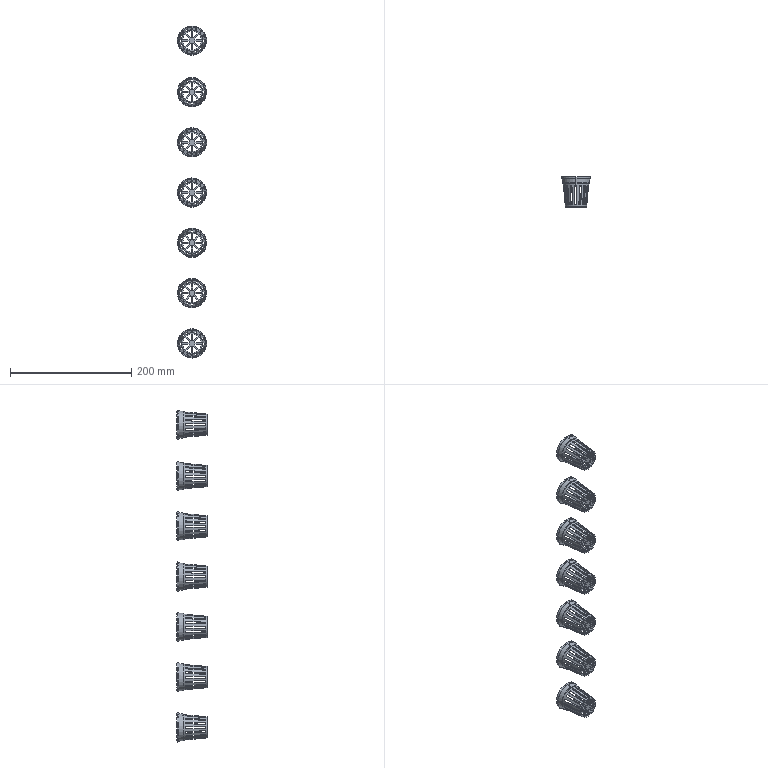Part | SolidWorks | 7 solids | 791 faces | box 48.245 x 49.817 x 548.245 mm | volume 30830 mm3 | plane 595 | cylinder 112 | cone 84 | commonest cylinder face diameters 10.222 x56 30.787 x56